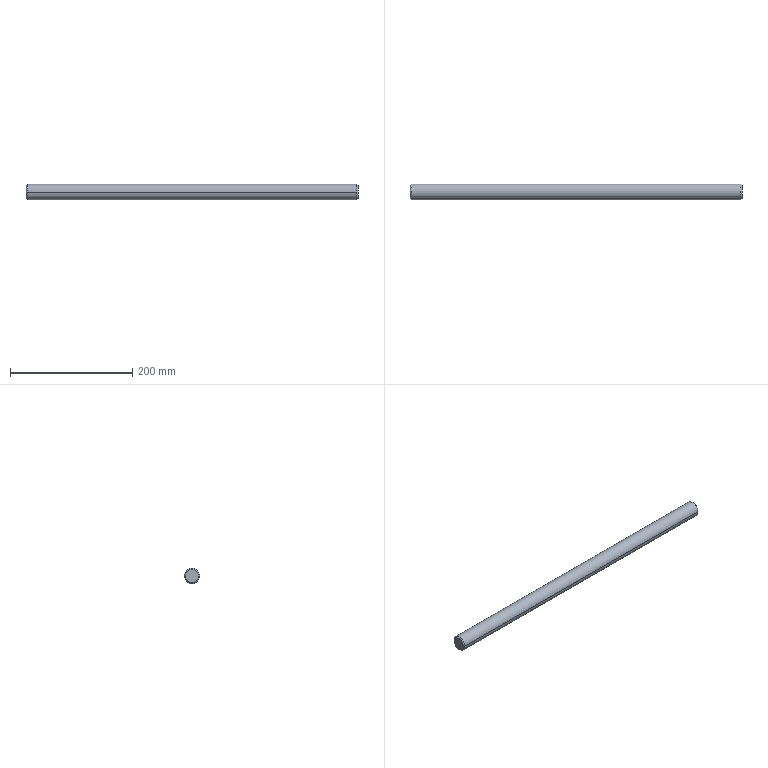Part | NX | features BREP 1 | 1 solid | 8 faces | box 542.798 x 25.4 x 25.4 mm | volume 274728 mm3 | cone 4 | plane 2 | cylinder 2 | commonest cylinder face diameters 25.4 x2
STEP:
#1=CARTESIAN_POINT('',(-271.399,10.668,0.));
#2=VERTEX_POINT('',#1);
#3=CARTESIAN_POINT('',(-271.399,-10.668,0.));
#4=VERTEX_POINT('',#3);
#5=CARTESIAN_POINT('',(-271.399,0.,0.));
#6=DIRECTION('',(1.,0.,0.));
#7=DIRECTION('',(0.,1.,0.));
#8=AXIS2_PLACEMENT_3D('',#5,#6,#7);
#9=CIRCLE('',#8,10.668);
#10=EDGE_CURVE('',#2,#4,#9,.T.);
#11=ORIENTED_EDGE('',*,*,#10,.F.);
#12=CARTESIAN_POINT('',(-271.399,0.,0.));
#13=DIRECTION('',(1.,0.,0.));
#14=DIRECTION('',(0.,-1.,0.));
#15=AXIS2_PLACEMENT_3D('',#12,#13,#14);
#16=CIRCLE('',#15,10.668);
#17=EDGE_CURVE('',#4,#2,#16,.T.);
#18=ORIENTED_EDGE('',*,*,#17,.F.);
#19=EDGE_LOOP('',(#11,#18));
#20=FACE_BOUND('',#19,.T.);
#21=CARTESIAN_POINT('',(-271.399,0.,0.));
#22=DIRECTION('',(1.,0.,0.));
#23=DIRECTION('',(0.,1.,0.));
#24=AXIS2_PLACEMENT_3D('',#21,#22,#23);
#25=PLANE('',#24);
#26=ADVANCED_FACE('',(#20),#25,.F.);
#27=CARTESIAN_POINT('',(-269.367,12.7,0.));
#28=VERTEX_POINT('',#27);
#29=CARTESIAN_POINT('',(-271.399,10.668,0.));
#30=DIRECTION('',(0.7071,0.7071,0.));
#31=VECTOR('',#30,1000.);
#32=LINE('',#29,#31);
#33=EDGE_CURVE('',#28,#2,#32,.F.);
#34=ORIENTED_EDGE('',*,*,#33,.F.);
#35=CARTESIAN_POINT('',(-269.367,-12.7,0.));
#36=VERTEX_POINT('',#35);
#37=CARTESIAN_POINT('',(-269.367,0.,0.));
#38=DIRECTION('',(1.,0.,0.));
#39=DIRECTION('',(0.,-1.,0.));
#40=AXIS2_PLACEMENT_3D('',#37,#38,#39);
#41=CIRCLE('',#40,12.7);
#42=EDGE_CURVE('',#36,#28,#41,.T.);
#43=ORIENTED_EDGE('',*,*,#42,.F.);
#44=CARTESIAN_POINT('',(-271.399,-10.668,0.));
#45=DIRECTION('',(0.7071,-0.7071,0.));
#46=VECTOR('',#45,1000.);
#47=LINE('',#44,#46);
#48=EDGE_CURVE('',#36,#4,#47,.F.);
#49=ORIENTED_EDGE('',*,*,#48,.T.);
#50=ORIENTED_EDGE('',*,*,#17,.T.);
#51=EDGE_LOOP('',(#34,#43,#49,#50));
#52=FACE_BOUND('',#51,.T.);
#53=CARTESIAN_POINT('',(-270.383,0.,0.));
#54=DIRECTION('',(1.,0.,0.));
#55=DIRECTION('',(0.,-1.,0.));
#56=AXIS2_PLACEMENT_3D('',#53,#54,#55);
#57=CONICAL_SURFACE('',#56,11.684,0.7854);
#58=ADVANCED_FACE('',(#52),#57,.T.);
#59=ORIENTED_EDGE('',*,*,#48,.F.);
#60=CARTESIAN_POINT('',(-269.367,0.,0.));
#61=DIRECTION('',(1.,0.,0.));
#62=DIRECTION('',(0.,1.,0.));
#63=AXIS2_PLACEMENT_3D('',#60,#61,#62);
#64=CIRCLE('',#63,12.7);
#65=EDGE_CURVE('',#28,#36,#64,.T.);
#66=ORIENTED_EDGE('',*,*,#65,.F.);
#67=ORIENTED_EDGE('',*,*,#33,.T.);
#68=ORIENTED_EDGE('',*,*,#10,.T.);
#69=EDGE_LOOP('',(#59,#66,#67,#68));
#70=FACE_BOUND('',#69,.T.);
#71=CARTESIAN_POINT('',(-270.383,0.,0.));
#72=DIRECTION('',(1.,0.,0.));
#73=DIRECTION('',(0.,-1.,0.));
#74=AXIS2_PLACEMENT_3D('',#71,#72,#73);
#75=CONICAL_SURFACE('',#74,11.684,0.7854);
#76=ADVANCED_FACE('',(#70),#75,.T.);
#77=CARTESIAN_POINT('',(269.367,-12.7,0.));
#78=VERTEX_POINT('',#77);
#79=CARTESIAN_POINT('',(-269.367,-12.7,0.));
#80=DIRECTION('',(1.,0.,0.));
#81=VECTOR('',#80,1000.);
#82=LINE('',#79,#81);
#83=EDGE_CURVE('',#36,#78,#82,.T.);
#84=ORIENTED_EDGE('',*,*,#83,.T.);
#85=CARTESIAN_POINT('',(269.367,12.7,0.));
#86=VERTEX_POINT('',#85);
#87=CARTESIAN_POINT('',(269.367,0.,0.));
#88=DIRECTION('',(1.,0.,0.));
#89=DIRECTION('',(0.,1.,0.));
#90=AXIS2_PLACEMENT_3D('',#87,#88,#89);
#91=CIRCLE('',#90,12.7);
#92=EDGE_CURVE('',#86,#78,#91,.T.);
#93=ORIENTED_EDGE('',*,*,#92,.F.);
#94=CARTESIAN_POINT('',(-269.367,12.7,0.));
#95=DIRECTION('',(1.,0.,0.));
#96=VECTOR('',#95,1000.);
#97=LINE('',#94,#96);
#98=EDGE_CURVE('',#28,#86,#97,.T.);
#99=ORIENTED_EDGE('',*,*,#98,.F.);
#100=ORIENTED_EDGE('',*,*,#65,.T.);
#101=EDGE_LOOP('',(#84,#93,#99,#100));
#102=FACE_BOUND('',#101,.T.);
#103=CARTESIAN_POINT('',(-271.399,0.,0.));
#104=DIRECTION('',(1.,0.,0.));
#105=DIRECTION('',(0.,-1.,0.));
#106=AXIS2_PLACEMENT_3D('',#103,#104,#105);
#107=CYLINDRICAL_SURFACE('',#106,12.7);
#108=ADVANCED_FACE('',(#102),#107,.T.);
#109=ORIENTED_EDGE('',*,*,#98,.T.);
#110=CARTESIAN_POINT('',(269.367,0.,0.));
#111=DIRECTION('',(1.,0.,0.));
#112=DIRECTION('',(0.,-1.,0.));
#113=AXIS2_PLACEMENT_3D('',#110,#111,#112);
#114=CIRCLE('',#113,12.7);
#115=EDGE_CURVE('',#78,#86,#114,.T.);
#116=ORIENTED_EDGE('',*,*,#115,.F.);
#117=ORIENTED_EDGE('',*,*,#83,.F.);
#118=ORIENTED_EDGE('',*,*,#42,.T.);
#119=EDGE_LOOP('',(#109,#116,#117,#118));
#120=FACE_BOUND('',#119,.T.);
#121=CARTESIAN_POINT('',(-271.399,0.,0.));
#122=DIRECTION('',(1.,0.,0.));
#123=DIRECTION('',(0.,-1.,0.));
#124=AXIS2_PLACEMENT_3D('',#121,#122,#123);
#125=CYLINDRICAL_SURFACE('',#124,12.7);
#126=ADVANCED_FACE('',(#120),#125,.T.);
#127=CARTESIAN_POINT('',(271.399,-10.668,0.));
#128=VERTEX_POINT('',#127);
#129=CARTESIAN_POINT('',(271.399,-10.668,0.));
#130=DIRECTION('',(-0.7071,-0.7071,0.));
#131=VECTOR('',#130,1000.);
#132=LINE('',#129,#131);
#133=EDGE_CURVE('',#128,#78,#132,.T.);
#134=ORIENTED_EDGE('',*,*,#133,.T.);
#135=ORIENTED_EDGE('',*,*,#115,.T.);
#136=CARTESIAN_POINT('',(271.399,10.668,0.));
#137=VERTEX_POINT('',#136);
#138=CARTESIAN_POINT('',(271.399,10.668,0.));
#139=DIRECTION('',(-0.7071,0.7071,0.));
#140=VECTOR('',#139,1000.);
#141=LINE('',#138,#140);
#142=EDGE_CURVE('',#137,#86,#141,.T.);
#143=ORIENTED_EDGE('',*,*,#142,.F.);
#144=CARTESIAN_POINT('',(271.399,0.,0.));
#145=DIRECTION('',(1.,0.,0.));
#146=DIRECTION('',(0.,-1.,0.));
#147=AXIS2_PLACEMENT_3D('',#144,#145,#146);
#148=CIRCLE('',#147,10.668);
#149=EDGE_CURVE('',#128,#137,#148,.T.);
#150=ORIENTED_EDGE('',*,*,#149,.F.);
#151=EDGE_LOOP('',(#134,#135,#143,#150));
#152=FACE_BOUND('',#151,.T.);
#153=CARTESIAN_POINT('',(270.383,0.,0.));
#154=DIRECTION('',(-1.,0.,0.));
#155=DIRECTION('',(0.,1.,0.));
#156=AXIS2_PLACEMENT_3D('',#153,#154,#155);
#157=CONICAL_SURFACE('',#156,11.684,0.7854);
#158=ADVANCED_FACE('',(#152),#157,.T.);
#159=CARTESIAN_POINT('',(271.399,0.,0.));
#160=DIRECTION('',(1.,0.,0.));
#161=DIRECTION('',(0.,1.,0.));
#162=AXIS2_PLACEMENT_3D('',#159,#160,#161);
#163=CIRCLE('',#162,10.668);
#164=EDGE_CURVE('',#137,#128,#163,.T.);
#165=ORIENTED_EDGE('',*,*,#164,.T.);
#166=ORIENTED_EDGE('',*,*,#149,.T.);
#167=EDGE_LOOP('',(#165,#166));
#168=FACE_BOUND('',#167,.T.);
#169=CARTESIAN_POINT('',(271.399,0.,0.));
#170=DIRECTION('',(1.,0.,0.));
#171=DIRECTION('',(0.,1.,0.));
#172=AXIS2_PLACEMENT_3D('',#169,#170,#171);
#173=PLANE('',#172);
#174=ADVANCED_FACE('',(#168),#173,.T.);
#175=ORIENTED_EDGE('',*,*,#142,.T.);
#176=ORIENTED_EDGE('',*,*,#92,.T.);
#177=ORIENTED_EDGE('',*,*,#133,.F.);
#178=ORIENTED_EDGE('',*,*,#164,.F.);
#179=EDGE_LOOP('',(#175,#176,#177,#178));
#180=FACE_BOUND('',#179,.T.);
#181=CARTESIAN_POINT('',(270.383,0.,0.));
#182=DIRECTION('',(-1.,0.,0.));
#183=DIRECTION('',(0.,1.,0.));
#184=AXIS2_PLACEMENT_3D('',#181,#182,#183);
#185=CONICAL_SURFACE('',#184,11.684,0.7854);
#186=ADVANCED_FACE('',(#180),#185,.T.);
#187=CLOSED_SHELL('',(#26,#58,#76,#108,#126,#158,#174,#186));
#188=MANIFOLD_SOLID_BREP('',#187);
#189=(LENGTH_UNIT()NAMED_UNIT(*)SI_UNIT(.MILLI.,.METRE.));
#190=UNCERTAINTY_MEASURE_WITH_UNIT(LENGTH_MEASURE(0.00001),#189,'','');
#191=(NAMED_UNIT(*)PLANE_ANGLE_UNIT()SI_UNIT($,.RADIAN.));
#192=(NAMED_UNIT(*)SI_UNIT($,.STERADIAN.)SOLID_ANGLE_UNIT());
#193=(GEOMETRIC_REPRESENTATION_CONTEXT(3)GLOBAL_UNCERTAINTY_ASSIGNED_CONTEXT((#190))GLOBAL_UNIT_ASSIGNED_CONTEXT((#189,#191,#192))REPRESENTATION_CONTEXT('',''));
#194=ADVANCED_BREP_SHAPE_REPRESENTATION('',(#188),#193);